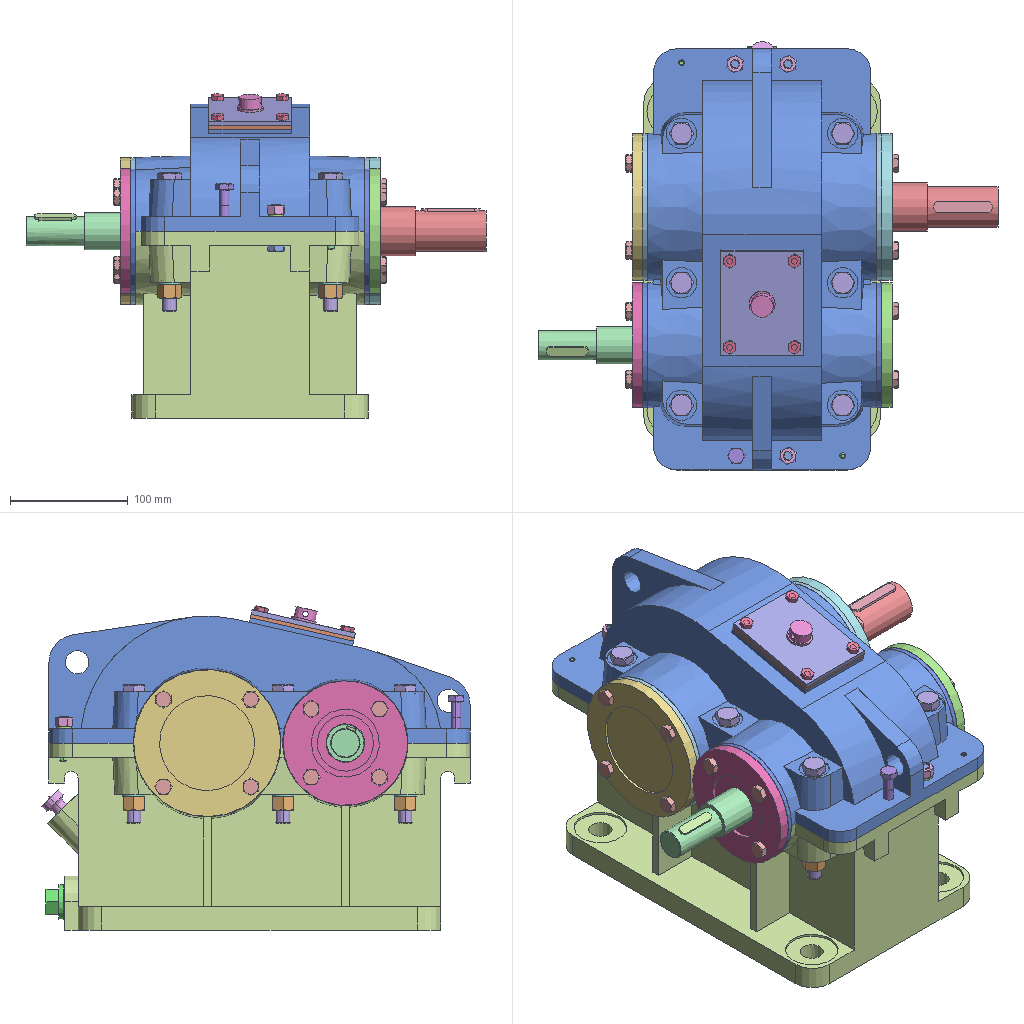Assembly | NX | 38 different items | 87 placed | box 391 x 364 x 276 mm
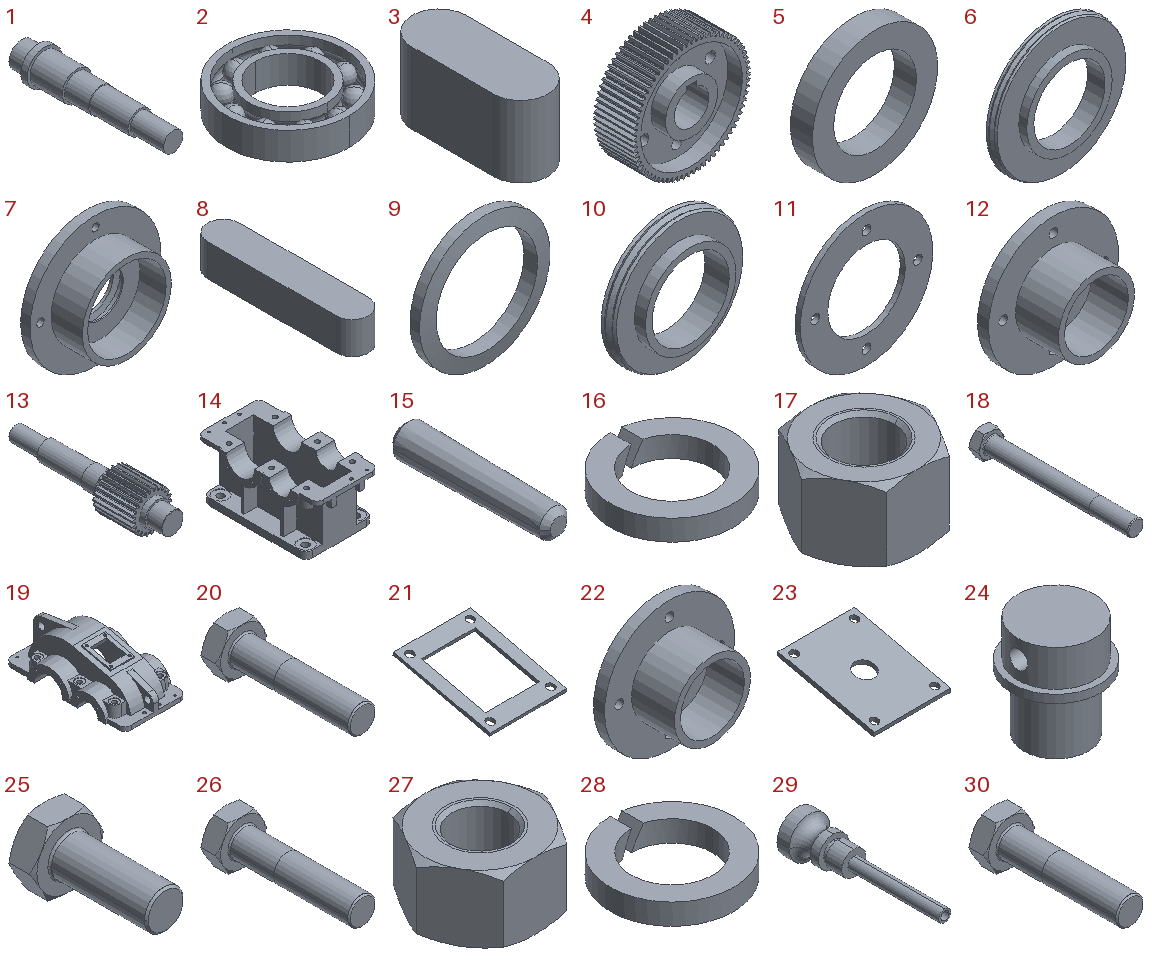Parts list (item | quantity | size | volume | features):
1 | x1 | 63 x 272 x 63 mm | 422770 mm3 | features DATUM_CSYS 9, EXTRUDE 8, SKETCH 8, BLEND 2
2 | x2 | 85 x 85 x 19 mm | 44629 mm3 | features BREP 12
3 | x1 | 16 x 40 x 21 mm | 12286 mm3 | features DATUM_CSYS 2, BLEND 1, EXTRUDE 1, OFFSET_REGION 1, SKETCH 1
4 | x1 | 180 x 60 x 179.897 mm | 648529 mm3 | features BREP 70, META 70, EXTRACT_DATUM_AXIS 14, DATUM_CSYS 10, EXTRUDE 9, SKETCH 9, EXTRACT_DATUM_PLANE 8, EXTRACT_STRING 8, Instance Feature 6, CYLINDER 1, FSET 1, Mirror Feature 1, Pattern Feature 1
5 | x1 | 68 x 12 x 68 mm | 24495 mm3 | features DATUM_CSYS 2, EXTRUDE 1, SKETCH 1
6 | x2 | 83.468 x 11 x 83.468 mm | 25904 mm3 | features DATUM_CSYS 5, SKETCH 4, EXTRUDE 3, SWP104 1
7 | x1 | 125 x 39 x 125 mm | 135227 mm3 | features DATUM_CSYS 8, HOLE PACKAGE 7, SIMPLE HOLE 7, SKETCH 7, EXTRACT_DATUM_AXIS 4, Instance Feature 3, EXTRUDE 2, Pattern Feature 1, SWP104 1
8 | x1 | 10 x 50 x 10 mm | 4785 mm3 | features DATUM_CSYS 2, BLEND 1, EXTRUDE 1, SKETCH 1
9 | x1 | 54 x 5.63 x 54 mm | 4326 mm3 | features DATUM_CSYS 2, SKETCH 1, SWP104 1
10 | x2 | 59.468 x 11 x 59.468 mm | 12056 mm3 | features DATUM_CSYS 5, SKETCH 4, EXTRUDE 3, SWP104 1
11 | x2 | 106 x 4 x 106 mm | 22607 mm3 | features DATUM_CSYS 6, HOLE PACKAGE 5, SIMPLE HOLE 5, SKETCH 5, EXTRACT_DATUM_AXIS 4, EXTRACT_FACE 4, Instance Feature 3, EXTRUDE 1, OFFSET_REGION 1, Pattern Feature 1
12 | x1 | 106 x 44 x 106 mm | 112067 mm3 | features DATUM_CSYS 7, HOLE PACKAGE 6, SIMPLE HOLE 6, SKETCH 6, EXTRACT_DATUM_AXIS 4, EXTRACT_FACE 4, Instance Feature 3, EXTRUDE 2, OFFSET_REGION 1, Pattern Feature 1
13 | x1 | 65 x 257 x 65 mm | 335559 mm3 | features BREP 24, META 24, DATUM_CSYS 8, EXTRUDE 7, SKETCH 7, EXTRACT_DATUM_AXIS 4, EXTRACT_DATUM_PLANE 2, EXTRACT_STRING 2, BLEND 1, CHAMFER 1, CYLINDER 1, FSET 1, Instance Feature 1, Mirror Feature 1
14 | x1 | 201 x 359.077 x 159 mm | 2835501 mm3 | features DATUM_CSYS 39, SIMPLE HOLE 38, SKETCH 38, EXTRACT_DATUM_AXIS 32, EXTRACT_FACE 26, HOLE PACKAGE 25, EXTRUDE 22, EXTRACT_DATUM_PLANE 14, Instance Feature 10, DRAFT 8, EXTRACT_STRING 8, BLEND 5, FSET 4, Mirror Feature 4, OFFSET_REGION 3, REPLACE_FACE 3, CPROJ 2, Pattern Feature 2, DATUM_PLANE 1
15 | x2 | 5.848 x 28 x 5.848 mm | 637.188 mm3 | features BREP 1
16 | x7 | 18.4 x 18.4 x 3.1 mm | 446.968 mm3 | features BREP 1
17 | x7 | 20.785 x 18 x 12.2 mm | 3340 mm3 | features BREP 2
18 | x7 | 20.785 x 117.5 x 18 mm | 15779 mm3 | features BREP 2
19 | x1 | 195 x 358 x 108 mm | 1561648 mm3 | features DATUM_CSYS 38, SIMPLE HOLE 38, SKETCH 37, EXTRACT_DATUM_AXIS 32, EXTRACT_FACE 26, HOLE PACKAGE 25, EXTRUDE 21, EXTRACT_DATUM_PLANE 14, Instance Feature 10, DRAFT 8, EXTRACT_STRING 8, BLEND 5, FSET 4, Mirror Feature 4, OFFSET_REGION 3, REPLACE_FACE 3, CPROJ 2, Pattern Feature 2, DATUM_PLANE 1, TRIM BODY 1
20 | x16 | 15.011 x 40.3 x 13 mm | 2917 mm3 | features BREP 2
21 | x1 | 70 x 88.433 x 22.841 mm | 9618 mm3 | features DATUM_CSYS 38, SIMPLE HOLE 38, SKETCH 37, EXTRACT_DATUM_AXIS 32, EXTRACT_FACE 26, HOLE PACKAGE 25, EXTRUDE 21, EXTRACT_DATUM_PLANE 14, Instance Feature 10, DRAFT 8, EXTRACT_STRING 8, BLEND 5, FSET 4, Mirror Feature 4, OFFSET_REGION 4, REPLACE_FACE 3, CPROJ 2, Pattern Feature 2, DATUM_PLANE 1, TRIM BODY 1
22 | x1 | 106 x 44 x 106 mm | 98017 mm3 | features DATUM_CSYS 8, HOLE PACKAGE 7, SIMPLE HOLE 7, SKETCH 7, EXTRACT_DATUM_AXIS 4, EXTRACT_FACE 4, Instance Feature 3, EXTRUDE 2, OFFSET_REGION 1, Pattern Feature 1, SWP104 1
23 | x1 | 70 x 88.654 x 23.816 mm | 23566 mm3 | features DATUM_CSYS 39, SIMPLE HOLE 38, SKETCH 38, EXTRACT_DATUM_AXIS 32, EXTRACT_FACE 26, HOLE PACKAGE 25, EXTRUDE 22, EXTRACT_DATUM_PLANE 14, Instance Feature 10, DRAFT 8, EXTRACT_STRING 8, BLEND 5, FSET 4, Mirror Feature 4, REPLACE_FACE 4, OFFSET_REGION 3, CPROJ 2, Pattern Feature 2, DATUM_PLANE 1, TRIM BODY 1
24 | x1 | 22 x 22 x 25 mm | 5690 mm3 | features DATUM_CSYS 6, EXTRUDE 5, SKETCH 5
25 | x4 | 11.547 x 19 x 10 mm | 976.022 mm3 | features BREP 2
26 | x3 | 15.011 x 40.3 x 13 mm | 2917 mm3 | features BREP 2
27 | x3 | 15.011 x 13 x 7.9 mm | 1139 mm3 | features BREP 2
28 | x3 | 12.3 x 12.3 x 2.1 mm | 136.667 mm3 | features BREP 1
29 | x1 | 20 x 74.367 x 20 mm | 5186 mm3 | features BREP 1
30 | x1 | 15.011 x 40.3 x 13 mm | 2917 mm3 | features BREP 2
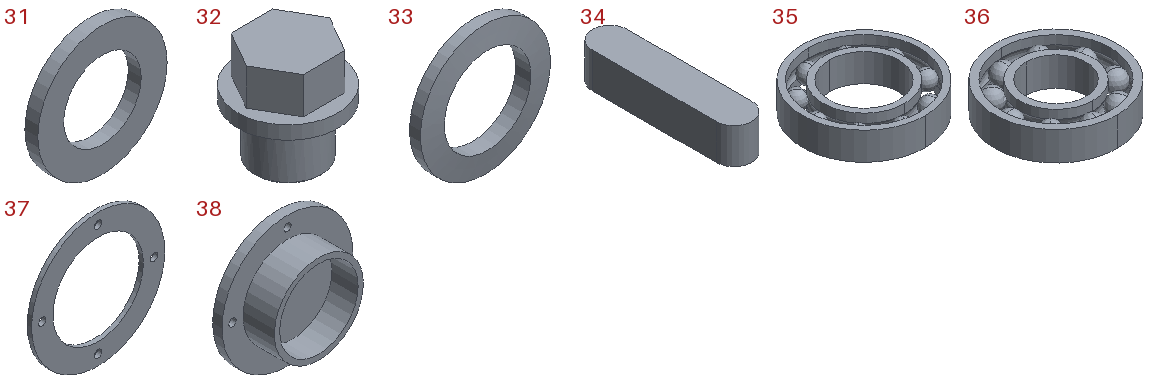31 | x1 | 30 x 3 x 30 mm | 1357 mm3 | features DATUM_CSYS 2, EXTRUDE 1, SKETCH 1
32 | x1 | 30 x 30 x 30 mm | 11818 mm3 | features DATUM_CSYS 5, EXTRUDE 4, SKETCH 4, CHAMFER 1
33 | x1 | 48 x 5.63 x 48 mm | 4786 mm3 | features DATUM_CSYS 2, SKETCH 1, SWP104 1
34 | x1 | 8 x 36 x 8 mm | 2194 mm3 | features DATUM_CSYS 2, BLEND 1, EXTRUDE 1, SKETCH 1
35 | x2 | 62 x 62 x 14 mm | 15463 mm3 | features BREP 11
36 | x1 | 72 x 72 x 17 mm | 30735 mm3 | features BREP 11
37 | x2 | 125 x 4 x 125 mm | 25774 mm3 | features DATUM_CSYS 2, EXTRUDE 1, SKETCH 1
38 | x1 | 125 x 39 x 125 mm | 158544 mm3 | features DATUM_CSYS 7, HOLE PACKAGE 6, SIMPLE HOLE 6, SKETCH 6, EXTRACT_DATUM_AXIS 4, Instance Feature 3, EXTRUDE 2, Pattern Feature 1
Mates (type | each side: item.copy, entity, surface, feature):
Fix | 14.1 component
Touch | 19.1 face cylinder Ø62 Hole(25) | 14.1 face cone Extrude(2)
Touch | 19.1 face cylinder Ø85 Hole(26) | 14.1 face cylinder Ø85 Hole(26)
Touch | 19.1 face plane Extrude(2) | 14.1 face plane Extrude(2)
Touch | 11.1 face cylinder Ø62 Hole(4) | 14.1 face cylinder Ø62 Hole(25)
Touch | 11.1 face cylinder Pattern Feature [Circular] (6) / Instance[3][0] | 14.1 face cylinder Pattern Feature [Circular] (48) / Instance[1][0]
Touch | 11.1 face plane Extrude(1) | 14.1 face plane Extrude(2)
Touch | 22.1 face cylinder Ø52 Hole(3) | 14.1 face cylinder Ø62 Hole(25) | 2 times
Touch | 11.1 face cylinder Extrude(1) | 14.1 face cylinder Ø62 Hole(25)
Touch | 11.1 face cylinder Pattern Feature [Circular] (6) / Instance[3][0] | 14.1 face cylinder Mirror Feature(50)
Touch | 11.1 face plane Extrude(1) | 14.1 face plane Mirror Feature(8)
Touch | 22.1 face cylinder Pattern Feature [Circular] (8) / Instance[1][0] | 14.1 face cylinder Mirror Feature(50)
Touch | 22.1 face plane Extrude(1) | 11.1 face plane Extrude(1)
Touch | 2.1 face cylinder Body(1) | 14.1 face cylinder Ø85 Hole(26)
Touch | 35.1 face cylinder Body(2) | 14.1 face cylinder Ø62 Hole(25)
Touch | 35.1 face plane Body(2) | 22.1 face plane Extrude(2)
Touch | 10.1 face cylinder Extrude(4) | 22.1 face cylinder Extrude(2)
Touch | 10.1 face plane Extrude(2) | 35.1 face plane Body(2)
Touch | 13.1 face cylinder Extrude(54) | 10.1 face cylinder Extrude(4)
Touch | 13.1 face plane Mirror Feature(53) | 10.1 face plane Extrude(1)
Touch | 10.1 face cylinder Extrude(4) | 13.1 face cylinder Extrude(52)
Touch | 10.1 face plane Extrude(1) | 13.1 face plane Extrude(51)
Touch | 35.1 face cylinder Body(1) | 13.1 face cylinder Extrude(52)
Touch | 35.1 face plane Body(2) | 10.1 face plane Extrude(2)
Touch | 12.1 face cylinder Ø52 Hole(3) | 35.1 face cylinder Body(1)
Touch | 12.1 face cylinder Pattern Feature [Circular] (7) / Instance[1][0] | 11.1 face cylinder Pattern Feature [Circular] (6) / Instance[3][0]
Touch | 12.1 face plane Extrude(1) | 11.1 face plane Extrude(1)
Touch | 37.1 face cylinder Extrude(1) | 14.1 face cylinder Ø85 Hole(26)
Touch | 37.1 face cylinder Extrude(1) | 14.1 face cylinder Mirror Feature(50)
Touch | 37.1 face plane Extrude(1) | 14.1 face plane Mirror Feature(8)
Touch | 38.1 face cylinder Extrude(2) | 14.1 face cylinder Ø85 Hole(26)
Touch | 38.1 face cylinder Pattern Feature [Circular] (5) / Instance[1][0] | 37.1 face cylinder Extrude(1)
Touch | 38.1 face plane Extrude(1) | 37.1 face plane Extrude(1)
Touch | 2.1 face plane Body(1) | 38.1 face plane Extrude(2)
Touch | 6.1 face cylinder Extrude(4) | 38.1 face cylinder Extrude(2)
Touch | 6.1 face plane Extrude(2) | 2.1 face plane Body(2)
Touch | 1.1 face cylinder Extrude(5) | 2.1 face cylinder Body(1)
Touch | 1.1 face plane Extrude(2) | 6.1 face plane Extrude(1)
Parallel | 1.1 face plane Extrude(7) | 14.1 face plane Extrude(11)
Touch | 8.1 face cylinder Edge Blend(2) | 1.1 face cylinder Edge Blend(8) | 2 times
Touch | 8.1 face plane Extrude(1) | 1.1 face plane Extrude(7)
Touch | 34.1 face cylinder Edge Blend(2) | 13.1 face cylinder Edge Blend(57) | 2 times
Touch | 34.1 face plane Extrude(1) | 13.1 face plane Extrude(56)
Touch | 3.1 face cylinder Edge Blend(2) | 1.1 face cylinder Edge Blend(10) | 2 times
Touch | 3.1 face plane Extrude(1) | 1.1 face plane Extrude(9)
Touch | 4.1 face cylinder Extrude(147) | 1.1 face cylinder Extrude(4)
Distance | 4.1 face plane Cylinder(1) | 1.1 face plane Extrude(2)
Touch | 5.1 face cylinder Extrude(1) | 4.1 face cylinder Extrude(143)
Touch | 5.1 face plane Extrude(1) | 4.1 face plane Cylinder(1)
Touch | 6.1 face cylinder Extrude(4) | 1.1 face cylinder Extrude(4)
Touch | 6.1 face plane Extrude(1) | 5.1 face plane Extrude(1)
Touch | 2.1 face cylinder Body(1) | 1.1 face cylinder Extrude(4)
Touch | 2.1 face plane Body(2) | 6.1 face plane Extrude(2)
Touch | 7.1 face cylinder Ø75 Hole(3) | 1.1 face cylinder Extrude(5)
Touch | 37.1 face cylinder Extrude(1) | 1.1 face cylinder Extrude(5)
Touch | 37.1 face plane Extrude(1) | 14.1 face plane Extrude(2)
Touch | 7.1 face cylinder Pattern Feature [Circular] (5) / Instance[3][0] | 37.1 face cylinder Extrude(1)
Touch | 7.1 face plane Extrude(1) | 37.1 face plane Extrude(1)
Touch | 21.1 face plane Extrude(18) | 19.1 face plane Extrude(18) | 2 times
Touch | 21.1 face plane Trim Body(73) | 19.1 face plane Extrude(18)
Touch | 23.1 face plane Extrude(18) | 21.1 face plane Extrude(18) | 2 times
Touch | 23.1 face plane Trim Body(51) | 21.1 face plane Extrude(18)
Touch | 24.1 face cylinder Extrude(4) | 23.1 face cylinder Extrude(53)
Touch | 24.1 face plane Extrude(2) | 23.1 face plane Extrude(18)
Touch | 25.1 face cylinder Body(1) | 23.1 face cylinder Extrude(18)
Touch | 25.1 face plane Body(1) | 23.1 face plane Extrude(18)
Bond | 23.1 component | assembly component | 2 times
Bond | 25.1 component | assembly component | 4 times
Linear2dPattern | assembly axis | assembly axis | assembly csys | assembly csys | assembly csys | assembly csys | 7 times
Touch | 29.1 face cylinder Body(1) | 14.1 face cylinder Edge Blend(15)
Touch | 29.1 face plane Body(1) | 14.1 face plane Ø17 Hole(27)
Touch | 31.1 face cylinder Extrude(1) | 14.1 face cylinder Ø20 Hole(29)
Touch | 31.1 face plane Extrude(1) | 14.1 face plane Ø31 Hole(30)
Touch | 32.1 face cylinder Extrude(4) | 14.1 face cylinder Edge Blend(17)
Touch | 32.1 face plane Extrude(2) | 31.1 face plane Extrude(1)
Touch | 15.1 face cone Body(1) | 19.1 face cylinder Extrude(36) | 2 times
Touch | 15.1 face plane Body(1) | 19.1 face plane Extrude(1) | 2 times
Touch | 18.1 face cylinder Body(1) | 19.1 face cylinder Extrude(31)
Touch | 18.1 face plane Body(1) | 19.1 face plane Ø26 Hole(32)
Touch | 16.1 face cylinder Body(1) | 18.1 face cylinder Body(1)
Touch | 16.1 face plane Body(1) | 14.1 face plane Ø26 Hole(33)
Touch | 17.1 face cylinder Body(1) | 18.1 face cylinder Body(1)
Touch | 17.1 face plane Body(1) | 16.1 face plane Body(1)
Bond | 19.1 component | assembly component | 6 times
Bond | 18.1 component | assembly component | 8 times
Bond | 17.1 component | assembly component | 8 times
Bond | 16.1 component | assembly component | 8 times
Touch | 30.1 face cylinder Body(1) | 19.1 face cylinder Extrude(36)
Touch | 30.1 face plane Body(1) | 14.1 face plane Extrude(36)
Touch | 26.1 face cylinder Body(1) | 14.1 face cylinder Extrude(36)
Touch | 26.1 face plane Body(1) | 14.1 face plane Extrude(1)
Touch | 28.1 face cylinder Body(1) | 26.1 face cylinder Body(1)
Touch | 28.1 face plane Body(1) | 19.1 face plane Extrude(1)
Touch | 27.1 face cylinder Body(1) | 26.1 face cylinder Body(1)
Touch | 27.1 face plane Body(1) | 28.1 face plane Body(1)
Bond | 26.1 component | assembly component | 4 times
Bond | 27.1 component | assembly component | 4 times
Bond | 28.1 component | assembly component | 4 times
LinearPattern | assembly axis | assembly csys | assembly csys | 6 times
Touch | 33.1 face cylinder Revolve(1) | 11.1 face cylinder Extrude(1)
Touch | 9.1 face cylinder Revolve(1) | 19.1 face cone Mirror Feature(8)
Touch | 20.1 face cylinder Body(1) | 12.1 face cylinder Pattern Feature [Circular] (7) / Instance[1][0]
Touch | 20.1 face plane Body(1) | 12.1 face plane Extrude(1)
Touch | 20.1 face cylinder Body(1) | 7.1 face cylinder Pattern Feature [Circular] (5) / Instance[3][0]
Touch | 20.1 face plane Body(1) | 7.1 face plane Extrude(1)
Touch | 20.1 face cylinder Body(1) | 38.1 face cylinder Ø7 Hole(4)
Touch | 20.1 face plane Body(1) | 38.1 face plane Extrude(1)
Touch | 20.1 face cylinder Body(1) | 22.1 face cylinder Ø7 Hole(7)
Touch | 20.1 face plane Body(1) | 22.1 face plane Extrude(1)
Fix | assembly component | 4 times
Bond | 20.1 component | assembly component | 16 times
CircularPattern | assembly axis | assembly csys | assembly csys | assembly csys | assembly csys | 4 times